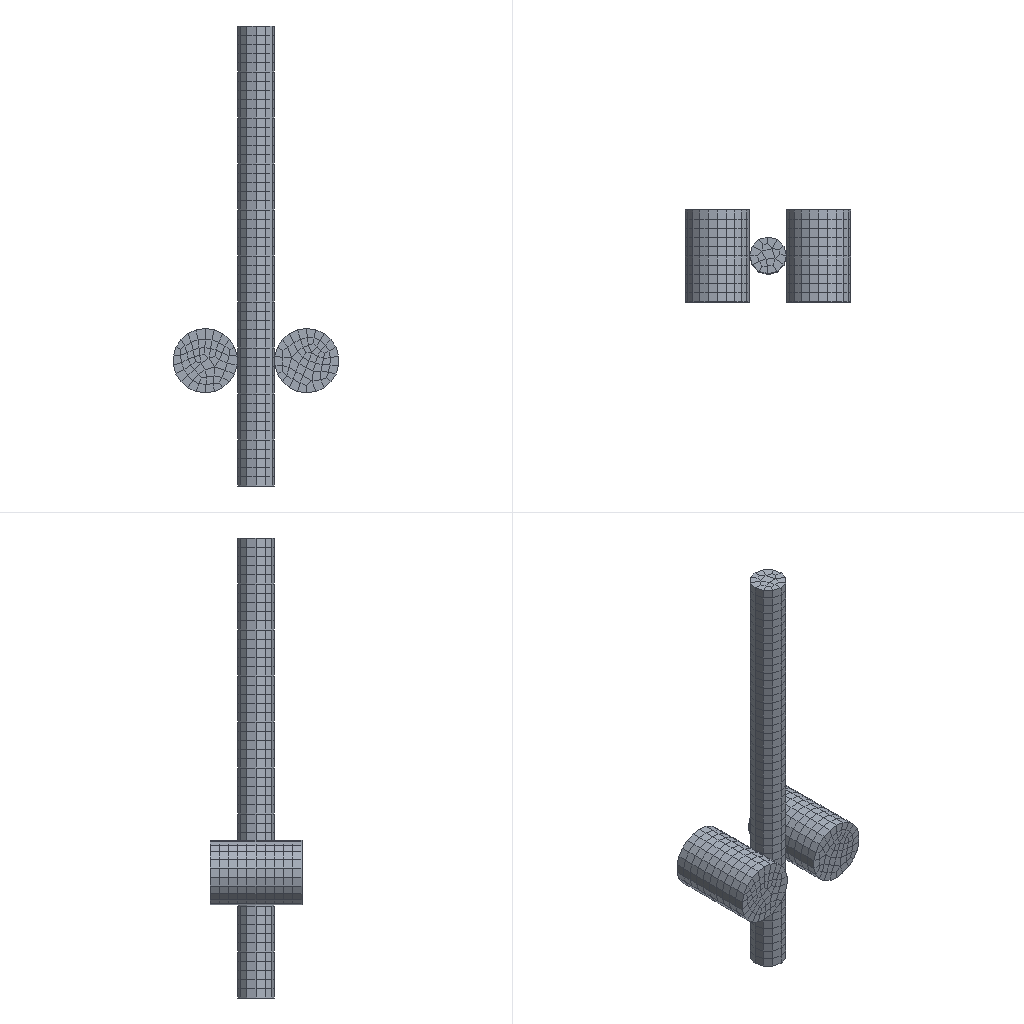Simulation study | abaqus
Set-up summary:
category,name,step,type,value,unit,region
solver,abaqus
solver,version,,,Abaqus/Explicit 2020
units,not stated in the deck,,not stated
analysis,deck,,transient,transient
load_step,Step-1,Step-1,transient
load_step,Step-2,Step-2,transient
load_step,requested,,,2
mesh,nodes,,,2760
mesh,elements,,,2010
element_type,C3D8R,,solid,2010
load,load commands in deck,,count,2
bc,support commands in deck,,count,14
material,MATERIAL-1,,in results
check,setup vs results,,match,"per instance, exact: element labels, types and connectivity; labels of the nodes the elements use; coordinates of those nodes at SINGLE_PRECISION in 3 of 3 instance(s)"
Abaqus input file, long lists of numbers shortened:
*Heading
** Job name: Job-1 Model name: Model-1
** Generated by: Abaqus/CAE 2020
*Preprint, echo=NO, model=NO, history=NO, contact=NO
**
** PARTS
**
*Part, name=work-1
*Node
      1, -0.454,          0.5,   1.698
      2, -0.3633,          0.5,   1.657
** (746 more lines like these left out)
*Element, type=C3D8R
  1,  24,  23,   1,  11,  92,  91,  69,  79
  2,  23,  25,   2,   1,  91,  93,  70,  69
** (558 more lines like these left out)
*Nset, nset=Set-1, generate
   1,  748,    1
*Elset, elset=Set-1, generate
   1,  560,    1
** Section: Section-1
*Solid Section, elset=Set-1, material=Material-1
,
*End Part
**
*Part, name=work-2
*Node
      1, -0.1732, -0.1,           0.
      2, -0.1, -0.1732,           0.
** (1273 more lines like these left out)
*Element, type=C3D8R
  1,   14,   24,    3,    4,   39,   49,   28,   29
  2,   25,    2,    3,   24,   50,   27,   28,   49
** (898 more lines like these left out)
*Nset, nset=Set-1, generate
    1,  1275,     1
*Elset, elset=Set-1, generate
   1,  900,    1
** Section: Section-1
*Solid Section, elset=Set-1, material=Material-1
,
*End Part
**
*Part, name=work-3
*Node
      1,  0.6496,          0.5,   1.698
      2,  0.7403,          0.5,   1.657
** (735 more lines like these left out)
*Element, type=C3D8R
  1,  24,  23,   1,  11,  91,  90,  68,  78
  2,  23,  25,   2,   1,  90,  92,  69,  68
** (548 more lines like these left out)
*Nset, nset=Set-1, generate
   1,  737,    1
*Elset, elset=Set-1, generate
   1,  550,    1
** Section: Section-1
*Solid Section, elset=Set-1, material=Material-1
,
*End Part
**
**
** ASSEMBLY
**
*Assembly, name=Assembly
**
*Instance, name=work-1-1, part=work-1
*End Instance
**
*Instance, name=work-2-1, part=work-2
*End Instance
**
*Instance, name=work-3-1, part=work-3
*End Instance
**
*Node
      1,   0.551,          0.5,   1.362
*Node
      2,   0.551,           0.,   1.362
*Nset, nset=Set-1, instance=work-2-1, generate
 1251,  1275,     1
*Elset, elset=Set-1, instance=work-2-1, generate
 883,  900,    1
*Nset, nset=Set-6
 2,
*Nset, nset=Set-7
 1,
*Nset, nset=b_Set-2, instance=work-3-1, generate
   1,  737,    1
*Elset, elset=b_Set-2, instance=work-3-1, generate
   1,  550,    1
*Nset, nset=b_Set-4, instance=work-1-1, generate
   1,  748,    1
*Elset, elset=b_Set-4, instance=work-1-1, generate
   1,  560,    1
*Nset, nset=_PickedSet16, internal
 1,
*Nset, nset=_PickedSet18, internal
 2,
*Elset, elset=_m_Surf-1_S5, internal, instance=work-1-1
   1,   2,  13,  15,  22,  24,  26,  29,  51,  54,  57,  58,  69,  71,  78,  80
  82,  85, 107, 110, 113, 114, 125, 127, 134, 136, 138, 141, 163, 166, 169, 170
** (5 more lines like these left out)
*Elset, elset=_m_Surf-1_S6, internal, instance=work-1-1
   4,   9,  60,  65, 116, 121, 172, 177, 228, 233, 284, 289, 340, 345, 396, 401
 452, 457, 508, 513
*Elset, elset=_m_Surf-1_S4, internal, instance=work-1-1
  16,  17,  18,  19,  20,  21,  28,  53,  72,  73,  74,  75,  76,  77,  84, 109
 128, 129, 130, 131, 132, 133, 140, 165, 184, 185, 186, 187, 188, 189, 196, 221
** (3 more lines like these left out)
*Elset, elset=_m_Surf-1_S3, internal, instance=work-1-1
   3,  52,  59, 108, 115, 164, 171, 220, 227, 276, 283, 332, 339, 388, 395, 444
 451, 500, 507, 556
*Surface, type=ELEMENT, name=m_Surf-1
_m_Surf-1_S5, S5
_m_Surf-1_S6, S6
_m_Surf-1_S4, S4
_m_Surf-1_S3, S3
*Elset, elset=_m_Surf-3_S5, internal, instance=work-3-1
   1,   2,  19,  21,  22,  31,  52,  53,  56,  57,  74,  76,  77,  86, 107, 108
 111, 112, 129, 131, 132, 141, 162, 163, 166, 167, 184, 186, 187, 196, 217, 218
** (3 more lines like these left out)
*Elset, elset=_m_Surf-3_S6, internal, instance=work-3-1
   4,  10,  17,  59,  65,  72, 114, 120, 127, 169, 175, 182, 224, 230, 237, 279
 285, 292, 334, 340, 347, 389, 395, 402, 444, 450, 457, 499, 505, 512
*Elset, elset=_m_Surf-3_S4, internal, instance=work-3-1
  23,  24,  25,  26,  28,  30,  54,  78,  79,  80,  81,  83,  85, 109, 133, 134
 135, 136, 138, 140, 164, 188, 189, 190, 191, 193, 195, 219, 243, 244, 245, 246
** (3 more lines like these left out)
*Elset, elset=_m_Surf-3_S3, internal, instance=work-3-1
   3,  27,  29,  32,  58,  82,  84,  87, 113, 137, 139, 142, 168, 192, 194, 197
 223, 247, 249, 252, 278, 302, 304, 307, 333, 357, 359, 362, 388, 412, 414, 417
** (1 more lines like these left out)
*Surface, type=ELEMENT, name=m_Surf-3
_m_Surf-3_S5, S5
_m_Surf-3_S6, S6
_m_Surf-3_S4, S4
_m_Surf-3_S3, S3
*Elset, elset=_s_Surf-1_S3, internal, instance=work-2-1
   5,   6,  14,  23,  24,  32,  41,  42,  50,  59,  60,  68,  77,  78,  86,  95
  96, 104, 113, 114, 122, 131, 132, 140, 149, 150, 158, 167, 168, 176, 185, 186
** (8 more lines like these left out)
*Elset, elset=_s_Surf-1_S4, internal, instance=work-2-1
   2,   8,   9,  15,  16,  20,  26,  27,  33,  34,  38,  44,  45,  51,  52,  56
  62,  63,  69,  70,  74,  80,  81,  87,  88,  92,  98,  99, 105, 106, 110, 116
** (14 more lines like these left out)
*Elset, elset=_s_Surf-1_S6, internal, instance=work-2-1
   3,  10,  21,  28,  39,  46,  57,  64,  75,  82,  93, 100, 111, 118, 129, 136
 147, 154, 165, 172, 183, 190, 201, 208, 219, 226, 237, 244, 255, 262, 273, 280
** (5 more lines like these left out)
*Elset, elset=_s_Surf-1_S5, internal, instance=work-2-1
   1,  11,  19,  29,  37,  47,  55,  65,  73,  83,  91, 101, 109, 119, 127, 137
 145, 155, 163, 173, 181, 191, 199, 209, 217, 227, 235, 245, 253, 263, 271, 281
** (5 more lines like these left out)
*Surface, type=ELEMENT, name=s_Surf-1
_s_Surf-1_S3, S3
_s_Surf-1_S4, S4
_s_Surf-1_S6, S6
_s_Surf-1_S5, S5
** Constraint: Constraint-1
*Rigid Body, ref node=_PickedSet16, elset=b_Set-2
** Constraint: Constraint-2
*Rigid Body, ref node=_PickedSet18, elset=b_Set-4
*End Assembly
*Amplitude, name=Amp-1
             0.,              0.,             0.1,              1.
**
** MATERIALS
**
*Material, name=Material-1
*Density
 7.8e-09,
*Elastic
191000., 0.29
*Plastic
1934.,0.
**
** INTERACTION PROPERTIES
**
*Surface Interaction, name=IntProp-1
*Friction
 0.2,
*Surface Behavior, pressure-overclosure=HARD
** ----------------------------------------------------------------
**
** STEP: Step-1
**
*Step, name=Step-1, nlgeom=YES
*Dynamic, Explicit
, 0.1
*Bulk Viscosity
0.06, 1.2
** Mass Scaling: Semi-Automatic
**               Whole Model
*Fixed Mass Scaling, factor=50.
**
** BOUNDARY CONDITIONS
**
** Name: BC-1 Type: 对称/反对称/完全固定
*Boundary
Set-1, ENCASTRE
** Name: BC-2 Type: 位移/转角
*Boundary, amplitude=Amp-1
Set-6, 1, 1
Set-6, 2, 2
Set-6, 3, 3
Set-6, 4, 4
Set-6, 5, 5, -0.4
Set-6, 6, 6
** Name: BC-3 Type: 对称/反对称/完全固定
*Boundary
Set-7, ENCASTRE
**
** INTERACTIONS
**
** Interaction: Int-1
*Contact Pair, interaction=IntProp-1, mechanical constraint=KINEMATIC, cpset=Int-1
m_Surf-1, s_Surf-1
** Interaction: Int-1-Copy
*Contact Pair, interaction=IntProp-1, mechanical constraint=KINEMATIC, cpset=Int-1-Copy
m_Surf-3, s_Surf-1
**
** OUTPUT REQUESTS
**
*Restart, write, number interval=1, time marks=NO
**
** FIELD OUTPUT: F-Output-1
**
*Output, field, variable=PRESELECT, number interval=50
*Output, history, frequency=0
*End Step
** ----------------------------------------------------------------
**
** STEP: Step-2
**
*Step, name=Step-2, nlgeom=YES
*Dynamic, Explicit
, 0.1
*Bulk Viscosity
0.06, 1.2
** Mass Scaling: Semi-Automatic
**               Whole Model
*Fixed Mass Scaling, factor=50.
**
** BOUNDARY CONDITIONS
**
** Name: BC-2 Type: 位移/转角
*Boundary, amplitude=Amp-1
Set-6, 1, 1
Set-6, 2, 2
Set-6, 3, 3
Set-6, 4, 4
Set-6, 5, 5, 0.4
Set-6, 6, 6
**
** OUTPUT REQUESTS
**
*Restart, write, number interval=1, time marks=NO
**
** FIELD OUTPUT: F-Output-1
**
*Output, field, number interval=50
*Node Output
A, CF, RF, RM, RT, U, UR, V
*Element Output, directions=YES
E, LE, MISES, MISESMAX, PE, PEEQ, PEMAG, S, SF
*Contact Output
CDISP, CSTRESS
*Output, history, frequency=0
*End Step
Results summary:
result,step,Step-1,completed,increments=1187111 time=0.1/0.1
result,step,Step-2,completed,increments=1187205 time=0.1/0.1
result,analysis,,,transient
result,last_loadstep,,,2
result,primary field,,,U
result,reaction total,,FX,0.000265,model units
result,reaction total,,FY,-0.000243,model units
result,reaction total,,FZ,-0.0232,model units